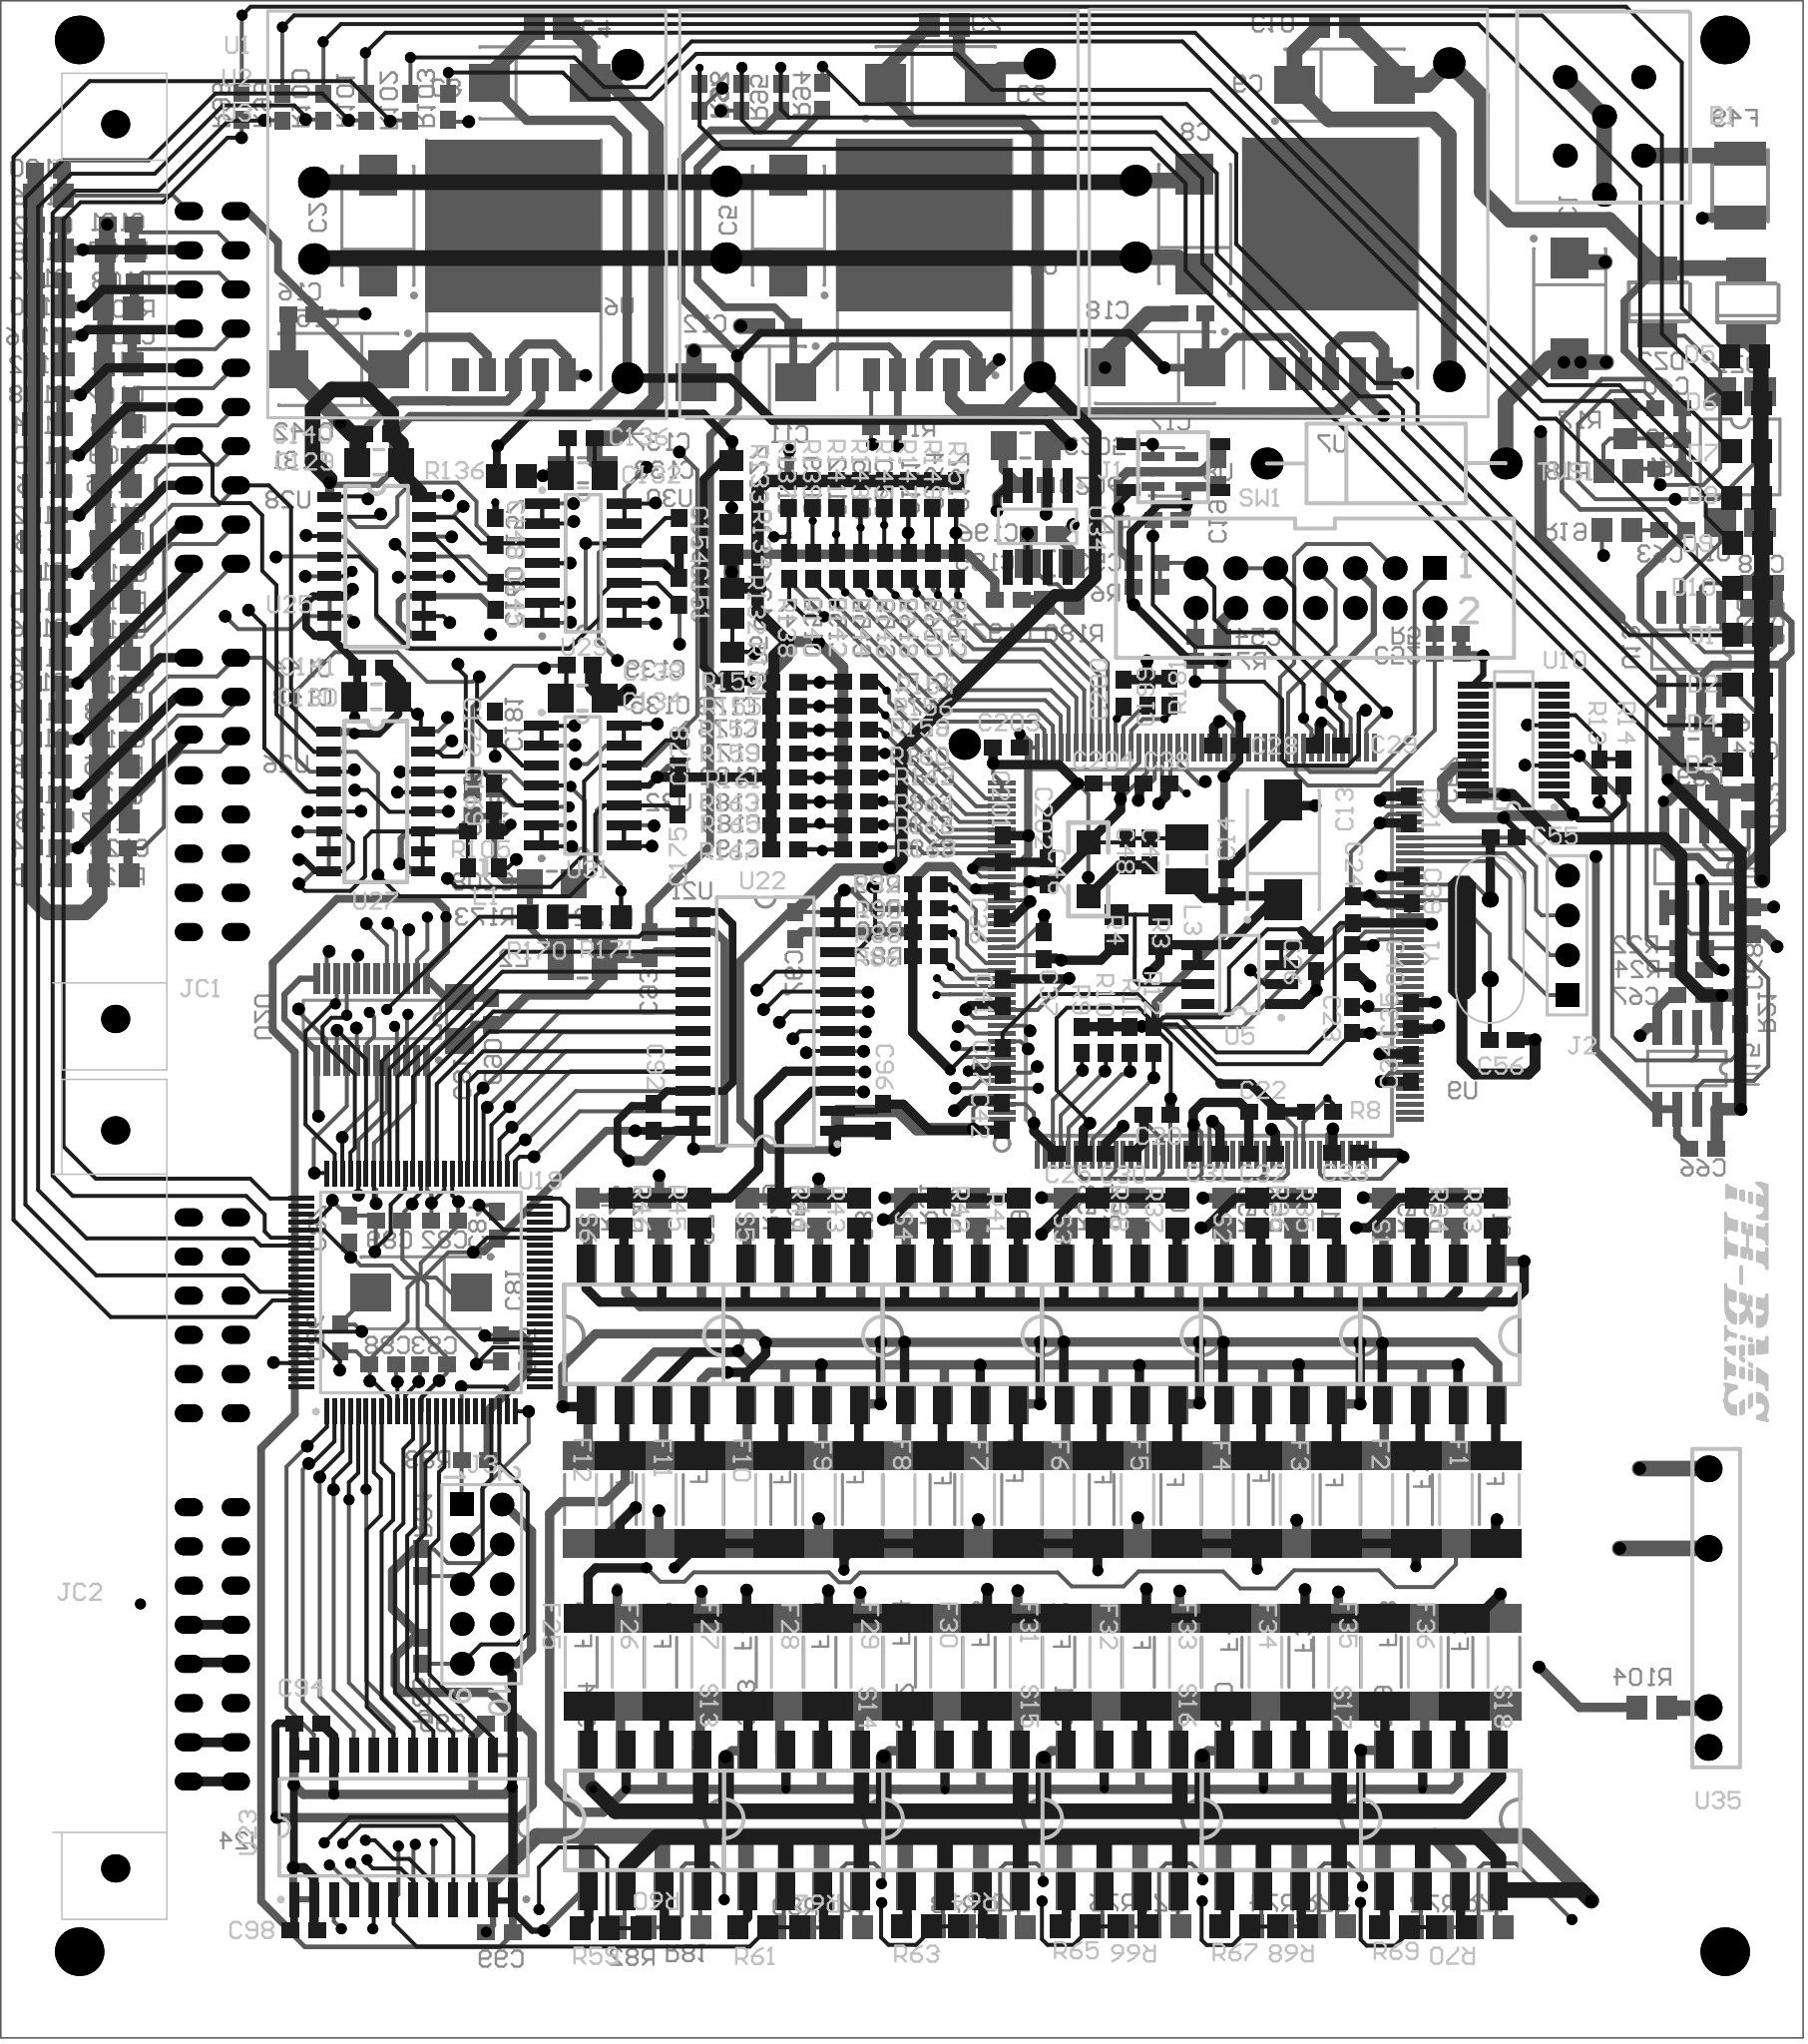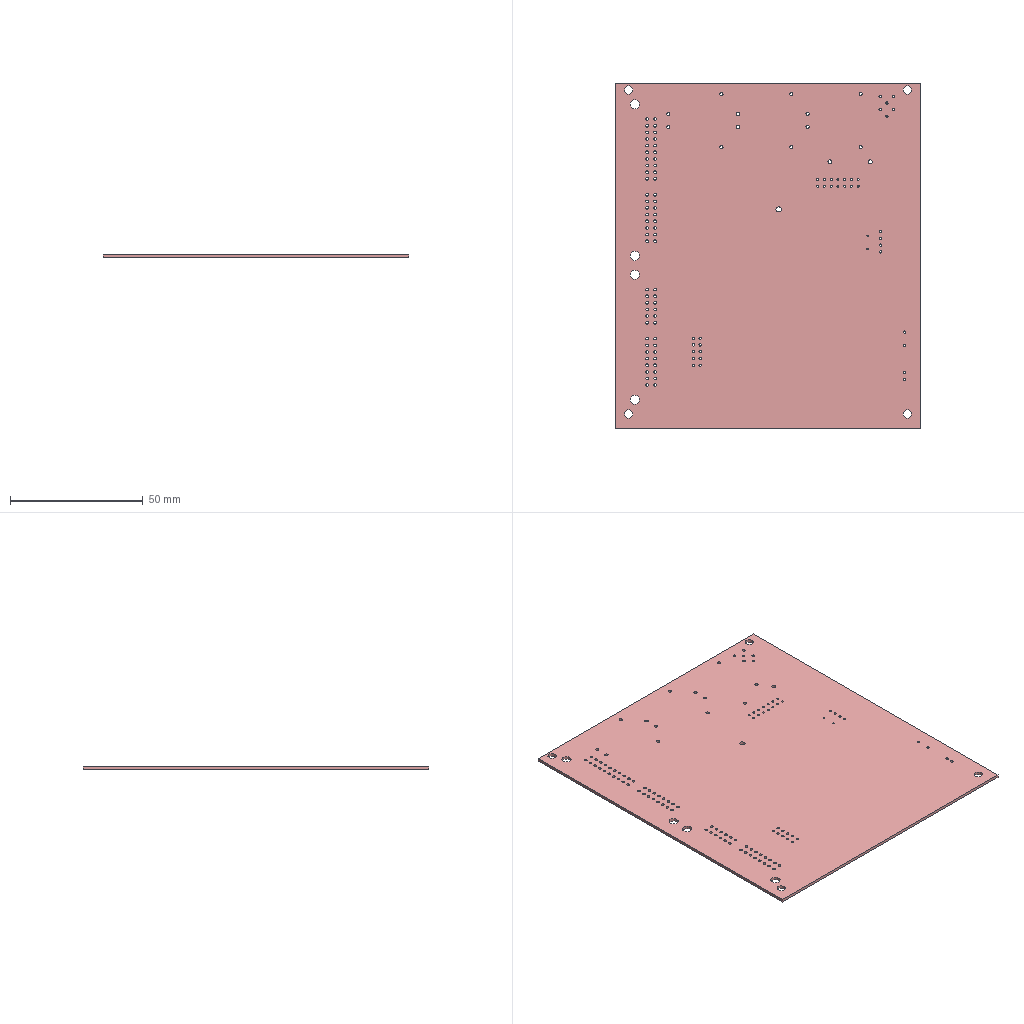Circuit board layout | Altium Designer | box 115 x 130 x 1.1 mm
Layer stack:
# Altium Designer layer stack of  (unit mm; dielectric type: 0 none, 1 core, 2 prepreg, 3 surface material)
index,name,kind,layer,copper_thickness_mm,dielectric_type,dielectric_thickness_mm,dielectric_material,dielectric_constant
0,Top Paste,other,,,,,,
1,Top Overlay,other,,,,,,
2,Top Solder,dielectric,,,3,0.0102,Solder Resist,3.5
3,Top Layer,copper,Top Layer,0.0356,,,,
4,Dielectric1,dielectric,,,1,0.32,FR-4,4.8
5,GND,copper,GND,0.0356,,,,
6,Dielectric2,dielectric,,,2,0.32,FR-4,4.8
7,POWER,copper,POWER,0.0356,,,,
8,Dielectric3,dielectric,,,1,0.32,FR-4,4.8
9,Bottom Layer,copper,Bottom Layer,0.0356,,,,
10,Bottom Solder,dielectric,,,3,0.0102,Solder Resist,3.5
11,Bottom Overlay,other,,,,,,
12,Bottom Paste,other,,,,,,
# drill layer pairs: low layer,high layer
drill_pair,Top Layer,Bottom Layer
Part placement:
Designator,Comment,Layer,Footprint,Center-X(mm),Center-Y(mm),Rotation
D1,RED,TopLayer,CR2012-0805,111.489,85.962,360
D2,RED,TopLayer,CR2012-0805,111.489,82.792,360
D3,GREEN,TopLayer,CR2012-0805,111.459,77.682,360
D4,GREEN,TopLayer,CR2012-0805,111.489,80.222,360
D5,BLUE,TopLayer,CR2012-0805,111.299,103.772,360
D6,BLUE,TopLayer,CR2012-0805,111.389,100.752,360
D7,BLUE,TopLayer,CR2012-0805,111.409,97.732,360
D8,BLUE,TopLayer,CR2012-0805,111.429,94.742,360
D9,BLUE,TopLayer,CR2012-0805,111.449,91.842,360
D10,RED,TopLayer,CR2012-0805,111.469,88.952,360
C55,Cap,TopLayer,CR1608-0603,95.9,73.062,180
C56,Cap,TopLayer,CR1608-0603,95.84,60.138,180
C199,Cap,TopLayer,CR1608-0603,73.152,82.3,270
C35,Cap,TopLayer,CR1608-0603,89.968,61.67,90
R181,Res2,TopLayer,CR1608-0603,74.548,82.32,90
C34,Cap,TopLayer,CR1608-0603,89.982,58.33,270
C38,Cap,TopLayer,CR1608-0603,73.74,76.502,360
R168,Res2,TopLayer,CR1608-0603,54.59,72.32,180
R166,Res2,TopLayer,CR1608-0603,54.59,73.844,180
R164,Res2,TopLayer,CR1608-0603,54.59,75.368,180
R162,Res2,TopLayer,CR1608-0603,54.59,76.892,180
R160,Res2,TopLayer,CR1608-0603,54.59,78.416,180
R158,Res2,TopLayer,CR1608-0603,54.59,79.94,180
R156,Res2,TopLayer,CR1608-0603,54.59,81.464,180
R154,Res2,TopLayer,CR1608-0603,54.59,82.988,180
R152,Res2,TopLayer,CR1608-0603,60.988,90.382,90
R150,Res2,TopLayer,CR1608-0603,59.464,90.382,90
R148,Res2,TopLayer,CR1608-0603,57.94,90.382,90
R146,Res2,TopLayer,CR1608-0603,56.416,90.382,90
R144,Res2,TopLayer,CR1608-0603,54.892,90.382,90
R142,Res2,TopLayer,CR1608-0603,53.368,90.382,90
R140,Res2,TopLayer,CR1608-0603,51.844,90.382,90
R138,Res2,TopLayer,CR1608-0603,50.32,90.382,90
C13,Cap Pol3,TopLayer,TC7343-2917,81.848,72.256,90
C14,Cap,TopLayer,CR1608-0603,78.212,70.17,270
R3,Res2,TopLayer,CR2012-0805,73.972,67.181,270
U22,SN74LVC4245PW,TopLayer,WSO24,48.792,61.314,90
B1,BNX012H,TopLayer,BNX012H,102.31,117.82,270
C20,Cap,TopLayer,CR1608-0603,73.79,55.372,360
C21,Cap,TopLayer,CR1608-0603,89.832,74.83,270
C22,Cap,TopLayer,CR1608-0603,80.51,55.542,360
C23,Cap,TopLayer,CR1608-0603,86.232,61.41,270
C24,Cap,TopLayer,CR1608-0603,86.262,68.45,270
C25,Cap,TopLayer,CR1608-0603,68.23,52.862,360
C26,Cap,TopLayer,CR1608-0603,83.928,65.35,90
C27,Cap,TopLayer,CR1608-0603,63.928,58.76,90
C28,Cap,TopLayer,CR1608-0603,78.25,78.902,360
C29,Cap,TopLayer,CR1608-0603,84.69,78.922,360
C30,Cap,TopLayer,CR1608-0603,71.37,52.868,180
C31,Cap,TopLayer,CR1608-0603,76.95,52.902,360
C32,Cap,TopLayer,CR1608-0603,80.49,52.902,360
C33,Cap,TopLayer,CR1608-0603,85.81,52.908,180
C36,Cap,TopLayer,CR1608-0603,63.882,68.762,270
C37,Cap,TopLayer,CR1608-0603,66.568,66.16,90
C39,Cap,TopLayer,CR1608-0603,90.058,69.72,90
C40,Cap,TopLayer,CR1608-0603,86.258,65.32,90
C41,Cap,TopLayer,CR1608-0603,63.918,63.174,90
C42,Cap,TopLayer,CR1608-0603,63.908,55.26,90
C46,Cap,TopLayer,1206,69.4,71.022,90
C47,Cap,TopLayer,CR1608-0603,73.308,72.13,90
C48,Cap,TopLayer,CR1608-0603,71.888,72.15,90
C92,Cap,TopLayer,CR1608-0603,41.662,55.18,270
C94,Cap,TopLayer,CR1608-0603,19.58,16.528,180
C96,Cap,TopLayer,CR1608-0603,56.272,55.18,270
C98,Cap,TopLayer,CR1608-0603,19.33,3.308,180
C129,Cap,TopLayer,CR3216-1206,24.139,96.992,360
C130,Cap,TopLayer,CR3216-1206,23.981,82.006,360
C132,Cap,TopLayer,CR3216-1206,37.165,96.162,180
C134,Cap,TopLayer,CR3216-1206,37.125,81.976,180
C136,Cap,TopLayer,CR1608-0603,37.054,98.564,180
C138,Cap,TopLayer,CR1608-0603,36.944,84.048,180
C140,Cap,TopLayer,CR1608-0603,24.07,98.798,360
C141,Cap,TopLayer,CR1608-0603,23.61,83.872,360
C145,Cap,TopLayer,CR1608-0603,31.604,88.426,90
C148,Cap,TopLayer,CR1608-0603,31.568,92.588,270
C151,Cap,TopLayer,CR1608-0603,43.282,88.746,270
C154,Cap,TopLayer,CR1608-0603,43.288,92.588,90
C169,Cap,TopLayer,CR1608-0603,31.488,75.66,90
C172,Cap,TopLayer,CR1608-0603,31.512,80.21,270
C175,Cap,TopLayer,CR1608-0603,43.212,75.36,270
C178,Cap,TopLayer,CR1608-0603,43.248,78.402,90
C200,Cap,TopLayer,CR1608-0603,71.672,82.28,270
C201,Cap,TopLayer,CR1608-0603,63.918,72.318,90
C202,Cap,TopLayer,CR1608-0603,66.792,70.89,270
C203,Cap,TopLayer,CR1608-0603,64.17,78.802,360
C204,Cap,TopLayer,CR1608-0603,70.61,76.492,360
F1,Res2,TopLayer,CR6332-2512,95.396,30.806,90
F2,Res2,TopLayer,CR6332-2512,90.316,30.806,90
F3,Res2,TopLayer,CR6332-2512,85.236,30.806,90
F4,Res2,TopLayer,CR6332-2512,80.156,30.806,90
F5,Res2,TopLayer,CR6332-2512,75.076,30.806,90
F6,Res2,TopLayer,CR6332-2512,69.996,30.806,90
F7,Res2,TopLayer,CR6332-2512,64.916,30.806,90
F8,Res2,TopLayer,CR6332-2512,59.836,30.806,90
F9,Res2,TopLayer,CR6332-2512,54.756,30.806,90
F10,Res2,TopLayer,CR6332-2512,49.676,30.806,90
F11,Res2,TopLayer,CR6332-2512,44.596,30.806,90
F12,Res2,TopLayer,CR6332-2512,39.516,30.806,90
F25,Res2,TopLayer,CR6332-2512,37.524,20.42,270
F26,Res2,TopLayer,CR6332-2512,42.604,20.42,270
F27,Res2,TopLayer,CR6332-2512,47.684,20.42,270
F28,Res2,TopLayer,CR6332-2512,52.764,20.42,270
F29,Res2,TopLayer,CR6332-2512,57.844,20.42,270
F30,Res2,TopLayer,CR6332-2512,62.924,20.42,270
F31,Res2,TopLayer,CR6332-2512,68.004,20.42,270
F32,Res2,TopLayer,CR6332-2512,73.084,20.42,270
F33,Res2,TopLayer,CR6332-2512,78.164,20.42,270
F34,Res2,TopLayer,CR6332-2512,83.244,20.42,270
F35,Res2,TopLayer,CR6332-2512,88.324,20.42,270
F36,Res2,TopLayer,CR6332-2512,93.404,20.42,270
J1,JTAG_335,TopLayer,JTAG14,83.866,88.963,180
J2,Header 4,TopLayer,HDR1X4,99.95,66.81,90
J3,JTAG_CPLD,TopLayer,HDR2X5,30.695,25.405,270
JC1,AMP-36P,TopLayer,36P,11.16,90.022,180
JC2,AMP-28P,TopLayer,28P,11.16,30.814,180
L3,Inductor,TopLayer,CR3225-1210,75.705,71.635,90
R4,Res2,TopLayer,CR2012-0805,71.188,67.169,90
R8,Res2,TopLayer,CR1608-0603,84.16,55.548,180
R9,Res2,TopLayer,CR1608-0603,68.998,60.126,90
R10,Res2,TopLayer,CR1608-0603,70.522,60.126,90
R11,Res2,TopLayer,CR1608-0603,72.046,60.126,90
R12,Res2,TopLayer,CR1608-0603,73.57,60.126,90
R13,Res2,TopLayer,CR1608-0603,102.022,77.21,270
R14,Res2,TopLayer,CR1608-0603,103.568,77.21,90
R33,Res2,TopLayer,CR2012-0805,95.414,49.103,90
R34,Res2,TopLayer,CR2012-0805,90.334,49.103,90
R35,Res2,TopLayer,CR2012-0805,84.746,49.103,90
R36,Res2,TopLayer,CR2012-0805,80.174,49.103,90
R37,Res2,TopLayer,CR2012-0805,75.094,49.103,90
R38,Res2,TopLayer,CR2012-0805,70.014,49.103,90
R41,Res2,TopLayer,CR2012-0805,64.934,49.103,90
R42,Res2,TopLayer,CR2012-0805,59.854,49.103,90
R43,Res2,TopLayer,CR2012-0805,54.774,49.103,90
R44,Res2,TopLayer,CR2012-0805,49.694,49.103,90
R45,Res2,TopLayer,CR2012-0805,44.614,49.103,90
R46,Res2,TopLayer,CR2012-0805,39.534,49.103,90
R59,Res2,TopLayer,CR2012-0805,37.899,3.452,360
R60,Res2,TopLayer,CR2012-0805,41.791,3.478,180
R61,Res2,TopLayer,CR2012-0805,47.969,3.502,360
R62,Res2,TopLayer,CR2012-0805,51.941,3.498,180
R63,Res2,TopLayer,CR2012-0805,58.429,3.562,360
R64,Res2,TopLayer,CR2012-0805,62.051,3.548,180
R65,Res2,TopLayer,CR2012-0805,68.579,3.562,360
R66,Res2,TopLayer,CR2012-0805,72.261,3.568,180
R67,Res2,TopLayer,CR2012-0805,78.729,3.552,360
R68,Res2,TopLayer,CR2012-0805,82.431,3.558,180
R69,Res2,TopLayer,CR2012-0805,88.939,3.512,360
R70,Res2,TopLayer,CR2012-0805,92.561,3.538,180
R86,Res2,TopLayer,CR1608-0603,59.05,65.482,360
R88,Res2,TopLayer,CR1608-0603,59.05,67.006,360
R90,Res2,TopLayer,CR1608-0603,59.05,68.53,360
R92,Res2,TopLayer,CR1608-0603,59.05,70.054,360
R131,Res2,TopLayer,CR2012-0805,46.686,83.951,90
R132,Res2,TopLayer,CR2012-0805,46.686,88.015,90
R133,Res2,TopLayer,CR2012-0805,46.65,96.125,270
R134,Res2,TopLayer,CR2012-0805,46.65,92.061,270
R136,Res2,TopLayer,CR2012-0805,32.611,96.126,360
R137,Res2,TopLayer,CR1608-0603,50.284,94.954,270
R139,Res2,TopLayer,CR1608-0603,51.808,94.954,270
R141,Res2,TopLayer,CR1608-0603,53.332,94.954,270
R143,Res2,TopLayer,CR1608-0603,54.856,94.954,270
R145,Res2,TopLayer,CR1608-0603,56.38,94.954,270
R147,Res2,TopLayer,CR1608-0603,57.904,94.954,270
R149,Res2,TopLayer,CR1608-0603,59.428,94.954,270
R151,Res2,TopLayer,CR1608-0603,60.952,94.954,270
R153,Res2,TopLayer,CR1608-0603,50.018,82.952,360
R155,Res2,TopLayer,CR1608-0603,50.018,81.428,360
R157,Res2,TopLayer,CR1608-0603,50.018,79.904,360
R159,Res2,TopLayer,CR1608-0603,50.018,78.38,360
R161,Res2,TopLayer,CR1608-0603,50.018,76.856,360
R163,Res2,TopLayer,CR1608-0603,50.018,75.332,360
R165,Res2,TopLayer,CR1608-0603,50.018,73.808,360
R167,Res2,TopLayer,CR1608-0603,50.018,72.284,360
R170,Res2,TopLayer,CR2012-0805,34.583,67.992,360
R171,Res2,TopLayer,CR2012-0805,38.647,67.992,360
S1,AQW214,TopLayer,AQW214,91.776,41.347,270
S2,AQW214,TopLayer,AQW214,81.617,41.347,270
S3,AQW214,TopLayer,AQW214,71.457,41.347,270
S4,AQW214,TopLayer,AQW214,61.297,41.347,270
S5,AQW214,TopLayer,AQW214,51.136,41.347,270
S6,AQW214,TopLayer,AQW214,40.977,41.347,270
S13,AQW214,TopLayer,AQW214,41.144,10.329,90
S14,AQW214,TopLayer,AQW214,51.303,10.329,90
S15,AQW214,TopLayer,AQW214,61.464,10.329,90
S16,AQW214,TopLayer,AQW214,71.624,10.329,90
S17,AQW214,TopLayer,AQW214,81.784,10.329,90
S18,AQW214,TopLayer,AQW214,91.944,10.329,90
SW1,SW-PB,TopLayer,SW_RESET,74.809,96.694,360
TVS1,1.5KE30A,TopLayer,SB560,88.405,96.92,180
U1,1205,TopLayer,DCDC_5W,29.981,112.368,0
U2,1205,TopLayer,DCDC_5W,56.271,112.428,0
U3,1205,TopLayer,DCDC_5W,82.405,112.478,0
U5,TPS76801Q,TopLayer,D008,79.038,64.305,90
U10,SN74CBTD3384DBLE,TopLayer,DBQ024,96.546,79.258,90
U19,EPM240T100C5N,TopLayer,TQFP100,26.816,44.014,90
U23,SN74LVC4245PW,TopLayer,WSO24,25.71,9.88,360
U25,MAX4619,TopLayer,SO16,23.991,90.355,0
U27,MAX4619,TopLayer,SO16,23.934,75.342,0
U29,OPA4350,TopLayer,751A-02,37.179,90.551,270
U31,OPA4350,TopLayer,751A-02,37.139,76.365,270
U34,ADR420,TopLayer,SO-G8,66.158,92.907,180
U35,AQZ102,TopLayer,AQZ102,108.956,23.875,90
Y1,30M,TopLayer,Oscillator,94.131,66.55,270
R105,Res2,TopLayer,CR1608-0603,30.66,73.448,180
L1,Inductor,TopLayer,INDC2012-0805,30.815,71.108,180
C192,Cap,BottomLayer,CR1608-0603,54.59,72.32,360
C189,Cap,BottomLayer,CR1608-0603,54.59,73.844,360
C186,Cap,BottomLayer,CR1608-0603,54.59,75.368,360
C183,Cap,BottomLayer,CR1608-0603,54.59,76.892,360
C180,Cap,BottomLayer,CR1608-0603,54.59,78.416,360
C177,Cap,BottomLayer,CR1608-0603,54.59,79.94,360
C174,Cap,BottomLayer,CR1608-0603,54.59,81.464,360
C171,Cap,BottomLayer,CR1608-0603,54.59,82.988,360
C168,Cap,BottomLayer,CR1608-0603,60.988,90.382,270
C165,Cap,BottomLayer,CR1608-0603,59.464,90.382,270
C162,Cap,BottomLayer,CR1608-0603,57.94,90.382,270
C159,Cap,BottomLayer,CR1608-0603,56.416,90.382,270
C156,Cap,BottomLayer,CR1608-0603,54.892,90.382,270
C153,Cap,BottomLayer,CR1608-0603,53.368,90.382,270
C150,Cap,BottomLayer,CR1608-0603,51.844,90.382,270
C147,Cap,BottomLayer,CR1608-0603,50.32,90.382,270
C89,Cap,BottomLayer,CR1608-0603,24.784,48.604,360
C81,Cap Pol3,BottomLayer,TC7343-2917,26.81,43.996,180
C82,Cap,BottomLayer,CR1608-0603,28.34,48.604,360
C87,Cap,BottomLayer,CR1608-0603,22.262,48.078,270
U21,SN74LVC4245PW,BottomLayer,WSO24,48.792,61.314,270
C15,Cap Pol3,BottomLayer,TC7343-2917,21.544,102.922,180
C16,Cap,BottomLayer,CR1608-0603,19.19,106.458,360
C17,Cap Pol3,BottomLayer,TC7343-2917,73.664,103.032,180
C18,Cap,BottomLayer,CR1608-0603,76.04,106.468,360
C19,Cap,BottomLayer,CR1608-0603,77.672,96.376,270
C52,Cap,BottomLayer,CR1608-0603,92.36,84.762,180
C53,Cap,BottomLayer,CR1608-0603,73.122,90.556,360
C54,Cap,BottomLayer,CR1608-0603,77.1,85.892,180
C58,Cap,BottomLayer,CR1608-0603,112.4,89.272,180
C59,Cap,BottomLayer,CR1608-0603,113.218,86.84,270
C60,Cap,BottomLayer,CR1608-0603,106.46,100.462,180
C61,Cap,BottomLayer,CR1608-0603,106.52,96.582,180
C62,Cap,BottomLayer,CR1608-0603,106.46,98.422,180
C63,Cap,BottomLayer,CR1608-0603,106.69,92.65,180
C83,Cap,BottomLayer,CR1608-0603,27.61,39.448,360
C84,Cap,BottomLayer,CR1608-0603,31.678,48.32,270
C85,Cap,BottomLayer,CR1608-0603,31.914,40.458,270
C86,Cap,BottomLayer,CR1608-0603,21.658,41.12,270
C88,Cap,BottomLayer,CR1608-0603,24.38,39.422,180
C90,Cap,BottomLayer,CR1608-0603,31.288,61.966,90
C91,Cap,BottomLayer,CR3216-1206,29.256,61.467,90
DZ1,SMBJ8.5CA,BottomLayer,AK_1B,111.36,107.171,180
DZ2,SMBJ8.5CA,BottomLayer,AK_1B,105.72,107.231,180
R5,Res2,BottomLayer,CR1608-0603,92.33,86.032,180
R6,Res2,BottomLayer,CR1608-0603,73.122,89.032,360
R7,Res2,BottomLayer,CR1608-0603,77.1,84.322,180
R17,Res2,BottomLayer,CR2012-0805,103.672,99.459,90
R18,Res2,BottomLayer,CR2012-0805,103.221,96.462,180
R19,Res2,BottomLayer,CR2012-0805,103.125,92.658,180
R83,Res2,BottomLayer,CR1608-0603,30.26,33.332,180
R84,Res2,BottomLayer,CR1608-0603,26.848,26.77,270
R85,Res2,BottomLayer,CR1608-0603,26.848,21.15,270
R104,Res2,BottomLayer,CR2012-0805,105.361,17.492,180
U8,TPS3823-33,BottomLayer,DBV005,74.587,96.385,90
U11,ZJYS-81R5-2PL,BottomLayer,ZJYS,110.993,97.335,90
U20,SN74CBTD3384DBLE,BottomLayer,DBQ024,23.688,61.442,180
R2,Res2,BottomLayer,CR1608-0603,74.39,93.332,180
C131,Cap,BottomLayer,CR3216-1206,24.129,97.008,360
C142,Cap,BottomLayer,CR1608-0603,24.07,98.834,360
C143,Cap,BottomLayer,CR3216-1206,23.981,82.042,360
C144,Cap,BottomLayer,CR1608-0603,23.59,83.868,360
U26,MAX4619,BottomLayer,SO16,23.941,75.345,180
U28,MAX4619,BottomLayer,SO16,23.998,90.352,180
C1,Cap Pol3,BottomLayer,TC7343-2917,100.118,106.824,270
C2,Cap Pol3,BottomLayer,TC7343-2917,24.072,112.09,90
C3,Cap Pol3,BottomLayer,TC7343-2917,34.386,121.208,360
C4,Cap,BottomLayer,CR2012-0805,34.971,124.712,180
F49,2.6A,BottomLayer,FUSE,110.991,114.649,270
C5,Cap Pol3,BottomLayer,TC7343-2917,50.272,112.1,90
C6,Cap Pol3,BottomLayer,TC7343-2917,59.656,121.228,360
C7,Cap,BottomLayer,CR2012-0805,60.201,124.892,180
C8,Cap Pol3,BottomLayer,TC7343-2917,76.192,112.2,90
C9,Cap Pol3,BottomLayer,TC7343-2917,85.756,121.068,360
C10,Cap,BottomLayer,CR2012-0805,85.131,124.812,180
C93,Cap,BottomLayer,CR1608-0603,41.382,66.18,90
C95,Cap,BottomLayer,CR1608-0603,31.81,16.488,360
C97,Cap,BottomLayer,CR1608-0603,50.692,67.43,90
C99,Cap,BottomLayer,CR1608-0603,31.83,3.208,360
C100,Cap,BottomLayer,CR1608-0603,3.05,115.598,360
C101,Cap,BottomLayer,CR1608-0603,7.66,112.188,360
C102,Cap,BottomLayer,CR1608-0603,3.079,112.136,360
C103,Cap,BottomLayer,CR1608-0603,7.689,108.566,360
C104,Cap,BottomLayer,CR1608-0603,3.12,108.618,360
C105,Cap,BottomLayer,CR1608-0603,7.54,105.018,360
C106,Cap,BottomLayer,CR1608-0603,3.12,105.088,360
C107,Cap,BottomLayer,CR1608-0603,7.44,101.278,360
C108,Cap,BottomLayer,CR1608-0603,3,101.318,360
C109,Cap,BottomLayer,CR1608-0603,7.4,97.418,360
C110,Cap,BottomLayer,CR1608-0603,2.96,97.458,360
C111,Cap,BottomLayer,CR1608-0603,7.4,93.638,360
C112,Cap,BottomLayer,CR1608-0603,2.87,93.608,360
C113,Cap,BottomLayer,CR1608-0603,7.32,89.888,360
C114,Cap,BottomLayer,CR1608-0603,2.89,89.918,360
C115,Cap,BottomLayer,CR1608-0603,7.3,86.25,360
C116,Cap,BottomLayer,CR1608-0603,2.86,86.316,360
C117,Cap,BottomLayer,CR1608-0603,7.25,82.812,360
C118,Cap,BottomLayer,CR1608-0603,2.92,82.898,360
C119,Cap,BottomLayer,CR1608-0603,7.26,79.334,360
C120,Cap,BottomLayer,CR1608-0603,2.94,79.31,360
C121,Cap,BottomLayer,CR1608-0603,7.269,75.814,360
C122,Cap,BottomLayer,CR1608-0603,2.97,75.822,360
C123,Cap,BottomLayer,CR1608-0603,7.28,72.358,360
C124,Cap,BottomLayer,CR1608-0603,2.98,72.398,360
F13,Res2,BottomLayer,CR6332-2512,37.484,30.806,90
F14,Res2,BottomLayer,CR6332-2512,42.056,30.806,90
F15,Res2,BottomLayer,CR6332-2512,47.644,30.806,90
F16,Res2,BottomLayer,CR6332-2512,52.216,30.806,90
F17,Res2,BottomLayer,CR6332-2512,57.804,30.806,90
F18,Res2,BottomLayer,CR6332-2512,62.376,30.806,90
F19,Res2,BottomLayer,CR6332-2512,67.964,30.806,90
F20,Res2,BottomLayer,CR6332-2512,72.536,30.806,90
F21,Res2,BottomLayer,CR6332-2512,78.124,30.806,90
F22,Res2,BottomLayer,CR6332-2512,82.696,30.806,90
F23,Res2,BottomLayer,CR6332-2512,88.284,30.806,90
F24,Res2,BottomLayer,CR6332-2512,92.856,30.806,90
F37,Res2,BottomLayer,CR6332-2512,95.436,20.42,270
F38,Res2,BottomLayer,CR6332-2512,90.864,20.42,270
F39,Res2,BottomLayer,CR6332-2512,85.276,20.42,270
F40,Res2,BottomLayer,CR6332-2512,80.704,20.42,270
F41,Res2,BottomLayer,CR6332-2512,75.116,20.42,270
F42,Res2,BottomLayer,CR6332-2512,70.036,20.42,270
F43,Res2,BottomLayer,CR6332-2512,64.956,20.42,270
F44,Res2,BottomLayer,CR6332-2512,59.876,20.42,270
F45,Res2,BottomLayer,CR6332-2512,54.796,20.42,270
F46,Res2,BottomLayer,CR6332-2512,49.716,20.42,270
F47,Res2,BottomLayer,CR6332-2512,44.636,20.42,270
F48,Res2,BottomLayer,CR6332-2512,39.556,20.42,270
R47,Res2,BottomLayer,CR2012-0805,37.466,49.103,90
R48,Res2,BottomLayer,CR2012-0805,42.038,49.103,90
R49,Res2,BottomLayer,CR2012-0805,47.626,49.103,90
R50,Res2,BottomLayer,CR2012-0805,52.198,49.103,90
R51,Res2,BottomLayer,CR2012-0805,57.786,49.103,90
R52,Res2,BottomLayer,CR2012-0805,62.358,49.103,90
R53,Res2,BottomLayer,CR2012-0805,67.946,49.103,90
R54,Res2,BottomLayer,CR2012-0805,72.518,49.103,90
R55,Res2,BottomLayer,CR2012-0805,78.106,49.103,90
R56,Res2,BottomLayer,CR2012-0805,82.678,49.103,90
R57,Res2,BottomLayer,CR2012-0805,88.266,49.103,90
R58,Res2,BottomLayer,CR2012-0805,92.838,49.103,90
R71,Res2,BottomLayer,CR2012-0805,94.941,3.542,180
R72,Res2,BottomLayer,CR2012-0805,91.089,3.508,360
R73,Res2,BottomLayer,CR2012-0805,84.841,3.592,180
R74,Res2,BottomLayer,CR2012-0805,80.889,3.568,360
R75,Res2,BottomLayer,CR2012-0805,74.341,3.552,180
R76,Res2,BottomLayer,CR2012-0805,70.709,3.548,360
R77,Res2,BottomLayer,CR2012-0805,64.451,3.542,180
R78,Res2,BottomLayer,CR2012-0805,60.589,3.558,360
R79,Res2,BottomLayer,CR2012-0805,54.021,3.532,180
R80,Res2,BottomLayer,CR2012-0805,50.439,3.488,360
R81,Res2,BottomLayer,CR2012-0805,43.751,3.492,180
R82,Res2,BottomLayer,CR2012-0805,40.239,3.498,360
R106,Res2,BottomLayer,CR2012-0805,3.041,114.012,180
R107,Res2,BottomLayer,CR2012-0805,7.651,110.522,180
R108,Res2,BottomLayer,CR2012-0805,3.07,110.51,180
R109,Res2,BottomLayer,CR2012-0805,7.53,106.81,180
R110,Res2,BottomLayer,CR2012-0805,3.111,106.932,180
R111,Res2,BottomLayer,CR2012-0805,7.531,103.272,180
R112,Res2,BottomLayer,CR2012-0805,3.111,103.252,180
R113,Res2,BottomLayer,CR2012-0805,7.431,99.282,180
R114,Res2,BottomLayer,CR2012-0805,2.991,99.422,180
R115,Res2,BottomLayer,CR2012-0805,7.391,95.502,180
R116,Res2,BottomLayer,CR2012-0805,2.951,95.502,180
R117,Res2,BottomLayer,CR2012-0805,7.321,91.922,180
R118,Res2,BottomLayer,CR2012-0805,2.861,91.922,180
R119,Res2,BottomLayer,CR2012-0805,7.311,88.082,180
R120,Res2,BottomLayer,CR2012-0805,2.881,88.172,180
R121,Res2,BottomLayer,CR2012-0805,7.311,84.492,180
R122,Res2,BottomLayer,CR2012-0805,2.901,84.492,180
R123,Res2,BottomLayer,CR2012-0805,7.231,81.122,180
R124,Res2,BottomLayer,CR2012-0805,2.931,81.102,180
R125,Res2,BottomLayer,CR2012-0805,7.271,77.572,180
R126,Res2,BottomLayer,CR2012-0805,2.911,77.582,180
R127,Res2,BottomLayer,CR2012-0805,7.28,74.11,180
R128,Res2,BottomLayer,CR2012-0805,2.951,74.162,180
R129,Res2,BottomLayer,CR2012-0805,7.271,70.642,180
R130,Res2,BottomLayer,CR2012-0805,2.935,70.618,180
S7,AQW214,BottomLayer,AQW214,41.103,41.347,270
S8,AQW214,BottomLayer,AQW214,51.264,41.347,270
S9,AQW214,BottomLayer,AQW214,61.423,41.347,270
S10,AQW214,BottomLayer,AQW214,71.584,41.347,270
S11,AQW214,BottomLayer,AQW214,81.743,41.347,270
S12,AQW214,BottomLayer,AQW214,91.903,41.347,270
S19,AQW214,BottomLayer,AQW214,91.817,10.329,90
S20,AQW214,BottomLayer,AQW214,81.656,10.329,90
S21,AQW214,BottomLayer,AQW214,71.496,10.329,90
S22,AQW214,BottomLayer,AQW214,61.337,10.329,90
S23,AQW214,BottomLayer,AQW214,51.176,10.329,90
S24,AQW214,BottomLayer,AQW214,41.017,10.329,90
U24,SN74LVC4245PW,BottomLayer,WSO24,25.704,9.892,180
C11,Cap Pol3,BottomLayer,TC7343-2917,47.554,102.102,180
C12,Cap,BottomLayer,CR1608-0603,49.73,105.688,360
C133,Cap,BottomLayer,CR3216-1206,37.161,96.482,180
C135,Cap,BottomLayer,CR3216-1206,37.125,81.94,180
C137,Cap,BottomLayer,CR1608-0603,37.054,98.528,180
C139,Cap,BottomLayer,CR1608-0603,36.944,84.012,180
C157,Cap,BottomLayer,CR1608-0603,31.604,92.588,270
C160,Cap,BottomLayer,CR1608-0603,31.568,88.426,90
C163,Cap,BottomLayer,CR1608-0603,43.252,92.588,90
C166,Cap,BottomLayer,CR1608-0603,43.318,88.746,270
C181,Cap,BottomLayer,CR1608-0603,31.524,80.222,270
C184,Cap,BottomLayer,CR1608-0603,31.502,75.32,90
C187,Cap,BottomLayer,CR1608-0603,43.212,78.402,90
R172,Res2,BottomLayer,CR2012-0805,38.629,67.992,180
R173,Res2,BottomLayer,CR2012-0805,34.611,68.052,180
U9,TMS320F283XXPGF_23,BottomLayer,QFP176NEW,76.889,65.793,90
U30,OPA4350,BottomLayer,751A-02,37.179,90.561,90
U32,OPA4350,BottomLayer,751A-02,37.139,76.375,90
C125,Cap,BottomLayer,CR2012-0805,46.686,83.933,270
C126,Cap,BottomLayer,CR2012-0805,46.686,87.997,270
C146,Cap,BottomLayer,CR1608-0603,50.32,94.954,270
C149,Cap,BottomLayer,CR1608-0603,51.844,94.954,270
C152,Cap,BottomLayer,CR1608-0603,53.368,94.954,270
C155,Cap,BottomLayer,CR1608-0603,54.892,94.954,270
C158,Cap,BottomLayer,CR1608-0603,56.416,94.954,270
C161,Cap,BottomLayer,CR1608-0603,57.94,94.954,270
C164,Cap,BottomLayer,CR1608-0603,59.464,94.954,270
C167,Cap,BottomLayer,CR1608-0603,60.988,94.954,270
C170,Cap,BottomLayer,CR1608-0603,50.018,82.988,360
C173,Cap,BottomLayer,CR1608-0603,50.018,81.464,360
C176,Cap,BottomLayer,CR1608-0603,50.018,79.94,360
C179,Cap,BottomLayer,CR1608-0603,50.018,78.416,360
C182,Cap,BottomLayer,CR1608-0603,50.018,76.892,360
C185,Cap,BottomLayer,CR1608-0603,50.018,75.368,360
C188,Cap,BottomLayer,CR1608-0603,50.018,73.844,360
C191,Cap,BottomLayer,CR1608-0603,50.018,72.32,360
R20,Res2,BottomLayer,CR1608-0603,111.508,86.84,270
R22,Res2,BottomLayer,CR1608-0603,107.92,65.982,180
R87,Res2,BottomLayer,CR1608-0603,59.05,65.482,180
R89,Res2,BottomLayer,CR1608-0603,59.05,67.006,180
R91,Res2,BottomLayer,CR1608-0603,59.05,68.53,180
R93,Res2,BottomLayer,CR1608-0603,59.05,70.054,180
R94,Res2,BottomLayer,CR1608-0603,52.442,120.332,90
R95,Res2,BottomLayer,CR1608-0603,49.788,120.302,90
R96,Res2,BottomLayer,CR1608-0603,44.61,120.302,90
R97,Res2,BottomLayer,CR1608-0603,47.256,120.292,90
R98,Res2,BottomLayer,CR1608-0603,15.386,119.704,90
R99,Res2,BottomLayer,CR1608-0603,17.972,119.664,90
R100,Res2,BottomLayer,CR1608-0603,20.598,119.664,90
R101,Res2,BottomLayer,CR1608-0603,23.294,119.664,90
R102,Res2,BottomLayer,CR1608-0603,26.15,119.664,90
R103,Res2,BottomLayer,CR1608-0603,28.556,119.674,90
U13,SN65HVD251,BottomLayer,D008,107.855,85.052,180
U15,HCPL063,BottomLayer,SO-G8,107.596,58.313,180
U16,HCPL063,BottomLayer,SO-G8,108.058,71.191,180
R1,Res2,BottomLayer,CR1608-0603,56.39,99.252,180
C127,Cap,BottomLayer,CR2012-0805,46.65,96.143,90
C128,Cap,BottomLayer,CR2012-0805,46.65,92.079,90
U4,TPS75733,BottomLayer,75733,58.947,107.339,180
U6,TPS75733,BottomLayer,75733,32.747,107.329,180
U7,TPS75733,BottomLayer,75733,84.867,107.439,180
C209,Cap,BottomLayer,CR1608-0603,30.102,75.27,90
C208,Cap,BottomLayer,CR3216-1206,35.169,70.098,360
C57,Cap,BottomLayer,CR1608-0603,93.968,76.68,270
C64,Cap,BottomLayer,CR3216-1206,108.021,78.542,180
C65,Cap,BottomLayer,CR1608-0603,107.8,80.382,180
C66,Cap,BottomLayer,CR1608-0603,108.61,53.218,360
C67,Cap,BottomLayer,CR1608-0603,107.85,62.968,360
C68,Cap,BottomLayer,CR1608-0603,111.802,67.76,90
C69,Cap,BottomLayer,CR1608-0603,108.51,75.928,360
C195,Cap,BottomLayer,CR3216-1206,66.941,90.552,180
C196,Cap,BottomLayer,CR1608-0603,66.42,92.442,180
C197,Cap,BottomLayer,CR1608-0603,64.28,88.228,360
C205,Cap,BottomLayer,CR3216-1206,65.379,98.068,360
C206,Cap,BottomLayer,CR1608-0603,65.84,95.548,360
L2,Inductor,BottomLayer,CR3225-1210,37.125,65.335,180
R21,Res2,BottomLayer,CR1608-0603,110.972,62.02,90
R23,Res2,BottomLayer,CR1608-0603,111.542,75.08,90
R24,Res2,BottomLayer,CR1608-0603,107.87,64.602,180
R180,Res2,BottomLayer,CR2012-0805,67.529,88.038,360
Pad and via stacks:
# Altium Designer via and pad stacks of  (unit mm). Each distinct definition once, with the count of objects using it.
# via: kind,start_layer,end_layer,hole_mm,diameter_mm,mode(0 simple;1 top-mid-bottom;2 full stack),diameter_per_layer,count,example_net
# pad: kind,layer,hole_mm,hole_type(0 round;1 square;2 slot),plating,top_size,top_shape(1 round;2 rect;3 octagon;9 rounded rect),mid_size,bottom_size,mode,footprint,size_per_layer,count,example
pad,Top Layer,0,0,plated,1.5x1.3,2,1.5x1.3,1.5x1.3,0,CR2012-0805,,86,D3.2
pad,Top Layer,0,0,plated,7.874x1.778,3,7.874x1.778,7.874x1.778,0,Oscillator,,1,Y1.3
pad,Top Layer,0,0,plated,1x1.1,2,1x1.1,1x1.1,0,CR1608-0603,,190,C55.1
pad,Top Layer,0,0,plated,2.6x2.4,2,2.6x2.4,2.6x2.4,0,TC7343-2917,,2,C13.1
pad,Top Layer,0,0,plated,2.7x1.6,2,2.7x1.6,2.7x1.6,0,CR3225-1210,,2,L3.1
pad,Top Layer,0,0,plated,0.4x1.95,2,0.4x1.95,0.4x1.95,0,DBQ024,,24,U10.13
pad,Top Layer,0,0,plated,0.6x2.2,2,0.6x2.2,0.6x2.2,0,WSO24,,48,U22.21
pad,Top Layer,0,0,plated,1.5x0.635,2,1.5x0.635,1.5x0.635,0,SO16,,32,U27.2
pad,Top Layer,0,0,plated,1.8x1.6,2,1.8x1.6,1.8x1.6,0,CR3216-1206,,8,C134.2
pad,Top Layer,0,0,plated,3.2x1.8,2,3.2x1.8,3.2x1.8,0,CR6332-2512,,48,F36.2
pad,Top Layer,0,0,plated,2.54x1.143,2,2.54x1.143,2.54x1.143,0,AQW214,,96,S18.1
pad,Top Layer,0,0,plated,0.6x2.2,2,0.6x2.2,0.6x2.2,0,SO-G8,,8,U34.3
pad,Top Layer,0,0,plated,0.6x2.2,2,0.6x2.2,0.6x2.2,0,751A-02,,28,U31.12
pad,Top Layer,0,0,plated,1.6x0.3,2,1.6x0.3,1.6x0.3,0,TQFP100,,100,U19.1
pad,Top Layer,0,0,plated,1.524x1.524,2,1.524x1.524,1.524x1.524,0,1206,,2,C46.2
pad,Top Layer,0,0,plated,1.524x0.762,2,1.524x0.762,1.524x0.762,0,SW_RESET,,4,SW1.4
pad,Top Layer,0,0,plated,0.6x2.05,2,0.6x2.05,0.6x2.05,0,D008,,8,U5.5
pad,Top Layer,0,0,plated,1.2x1,2,1.2x1,1.2x1,0,INDC2012-0805,,2,L1.1
pad,Bottom Layer,0,0,plated,1x1.1,2,1x1.1,1x1.1,0,CR1608-0603,,262,C209.1
pad,Bottom Layer,0,0,plated,1.8x1.6,2,1.8x1.6,1.8x1.6,0,CR3216-1206,,18,C208.2
pad,Bottom Layer,0,0,plated,2.7x1.6,2,2.7x1.6,2.7x1.6,0,CR3225-1210,,2,L2.2
pad,Bottom Layer,0,0,plated,1.5x1.3,2,1.5x1.3,1.5x1.3,0,CR2012-0805,,126,R180.1
pad,Bottom Layer,0,0,plated,1.778x0.3,2,1.778x0.3,1.778x0.3,0,QFP176NEW,,176,U9.53
pad,Bottom Layer,0,0,plated,0.6x2.2,2,0.6x2.2,0.6x2.2,0,WSO24,,48,U21.10
pad,Bottom Layer,0,0,plated,11.176x11,2,11.176x11,11.176x11,0,75733,,3,U7.6
pad,Bottom Layer,0,0,plated,1.05x2.1,2,1.05x2.1,1.05x2.1,0,75733,,15,U7.2
pad,Bottom Layer,0,0,plated,2.6x2.4,2,2.6x2.4,2.6x2.4,0,TC7343-2917,,22,C8.1
pad,Bottom Layer,0,0,plated,1.5x0.635,2,1.5x0.635,1.5x0.635,0,SO16,,32,U28.13
pad,Bottom Layer,0,0,plated,0.6x2.2,2,0.6x2.2,0.6x2.2,0,SO-G8,,16,U16.1
pad,Bottom Layer,0,0,plated,0.6x2.05,2,0.6x2.05,0.6x2.05,0,D008,,8,U13.1
pad,Bottom Layer,0,0,plated,0.6x2.2,2,0.6x2.2,0.6x2.2,0,751A-02,,28,U32.11
pad,Bottom Layer,0,0,plated,2.54x1.143,2,2.54x1.143,2.54x1.143,0,AQW214,,96,S24.8
pad,Bottom Layer,0,0,plated,3.2x1.8,2,3.2x1.8,3.2x1.8,0,CR6332-2512,,48,F48.1
pad,Bottom Layer,0,0,plated,1.524x3.302,2,1.524x3.302,1.524x3.302,0,FUSE,,2,F49.2
pad,Bottom Layer,0,0,plated,0.55x1.45,2,0.55x1.45,0.55x1.45,0,DBV005,,5,U8.1
pad,Bottom Layer,0,0,plated,0.4x1.95,2,0.4x1.95,0.4x1.95,0,DBQ024,,24,U20.1
pad,Bottom Layer,0,0,plated,1.524x2.54,2,1.524x2.54,1.524x2.54,0,AK_1B,,4,DZ2.2
pad,Bottom Layer,0,0,plated,1.8x2,2,1.8x2,1.8x2,0,ZJYS,,4,U11.4
pad,Multi-Layer,0.762,0,plated,1.524x1.524,1,1.524x1.524,1.524x1.524,0,JTAG14,,13,J1.7
pad,Multi-Layer,0.762,0,plated,1.524x1.524,2,1.524x1.524,1.524x1.524,0,JTAG14,,1,J1.1
pad,Multi-Layer,0.508,0,plated,1.016x1.016,1,1.016x1.016,1.016x1.016,0,Oscillator,,2,Y1.1
pad,Multi-Layer,1.2,0,plated,2x2,1,2x2,2x2,0,DCDC_5W,,12,U3.1
pad,Multi-Layer,1.397,0,plated,2.032x2.032,1,2.032x2.032,2.032x2.032,0,SB560,,2,TVS1.2
pad,Multi-Layer,1,0,plated,1.524x1.524,1,1.524x1.524,1.524x1.524,0,BNX012H,,4,B1.1
pad,Multi-Layer,0.9,0,plated,1.7x1.7,1,1.7x1.7,1.7x1.7,0,AQZ102,,4,U35.4
pad,Multi-Layer,0.9,0,plated,1.5x1.5,2,1.5x1.5,1.5x1.5,0,HDR1X4,,1,J2.1
pad,Multi-Layer,0.9,0,plated,1.5x1.5,1,1.5x1.5,1.5x1.5,0,HDR1X4,,3,J2.2
pad,Multi-Layer,0.9,0,plated,1.5x1.5,2,1.5x1.5,1.5x1.5,0,HDR2X5,,1,J3.1
pad,Multi-Layer,0.9,0,plated,1.5x1.5,1,1.5x1.5,1.5x1.5,0,HDR2X5,,9,J3.2
pad,Multi-Layer,0.8,0,plated,1.524x1.524,1,1.524x1.524,1.524x1.524,0,BNX012H,,2,B1.5
pad,Multi-Layer,3.1,0,plated,3.1x3.1,1,3.1x3.1,3.1x3.1,0,,,4,1
pad,Multi-Layer,1,0,plated,1.8x1.143,1,1.8x1.143,1.8x1.143,0,28P,,28,JC2.3
pad,Multi-Layer,3.5,0,plated,1.8x1.8,1,1.8x1.8,1.8x1.8,0,28P,,2,JC2.0
pad,Multi-Layer,1,0,plated,1.8x1.143,1,1.8x1.143,1.8x1.143,0,36P,,36,JC1.17
pad,Multi-Layer,3.5,0,plated,1.8x1.8,1,1.8x1.8,1.8x1.8,0,36P,,2,JC1.0
pad,Multi-Layer,2,0,plated,2x2,1,2x2,2x2,0,,,1,5
via,Top Layer,Bottom Layer,0.4,0.7,0,,83,BAT23
via,Top Layer,Bottom Layer,0.4,0.8,0,,339,BAT8
via,Top Layer,Bottom Layer,0.254,0.5,0,,37,NetC200_2
Copper pours:
name,layer,net,type(0 solid;1 hatched;2 none)
Top Layer-No Net,GND,GNDA,0
Top Layer-No Net,POWER,GNDD,0
Design rules, without the lines most boards share:
# Altium Designer design rules of  (exported by Altium Designer, unit mm)
# columns: name | kind | enabled | priority | scope1 | scope2 | descriptor | typed fields (field=value)
PlaneClearance | 12 | enabled | 1 | All | All | Power Plane Clearance (Clearance =0.508mm) (All) | clearance=0.508
PolygonConnect | 20 | enabled | 1 | All | All | Polygon Connect Rule(Relief Connect )(Conductor Width=0.254mm) (Relief Angle=90 Angle) (Entries=4) (Air Gap Width=0.254mm) (All),(All) | connect_style(0=relief,1=direct,2=none)=0 relief_conductor_width=0.254 relief_entries=4
PasteMaskExpansion | 14 | enabled | 1 | All | All | Paste Mask Expansion (Expansion =0mm) (All) | expansion=0
SolderMaskExpansion | 13 | enabled | 1 | All | All | Solder Mask Expansion (Expansion =0.102mm) (All) | expansion=0.1016
TestPointUsage | 44 | enabled | 1 | All | All | Fabrication Testpoint Usage (Valid =One Required, Allow multiple per net=No) (All) |
Testpoint | 43 | enabled | 1 | All | All | Fabrication Testpoint Style (Under Component=Yes) (All) |
ComponentClearance | 24 | enabled | 1 | All | All | Component Clearance Constraint ( Horizontal Gap = 0.254mm, Vertical Gap = 0.254mm ) (All),(All)  | gap=0.254
Height | 50 | enabled | 1 | All | All | Height Constraint (Min=0mm) (Max=25.4mm) (Prefered=12.7mm) (All) | min_height=0 max_height=25.4
HoleSize | 42 | enabled | 1 | All | All | Hole Size Constraint (Min=0.025mm) (Max=2.54mm) (All) |
Width | 2 | enabled | 1 | All | All | Width Constraint (Min=0.254mm) (Max=254mm) (Preferred=0.254mm) (All) |
Clearance | 0 | enabled | 1 | All | All | Clearance Constraint (Gap=0.3mm) (All),(All) | gap=0.3
RoutingCorners | 10 | enabled | 1 | All | All | Routing Corners (Style=45-Degree) (Min Setback=2.54mm) (Max Setback=2.54mm) (All) |
RoutingVias | 11 | enabled | 1 | All | All | Routing Via (MinHoleWidth=0.305mm) (MaxHoleWidth=5.08mm) (PreferredHoleWidth=0.381mm) (MinWidth=0.559mm) (MaxWidth=6.858mm) (PreferedWidth=0.762mm) (All) | via_min_hole=0.3048 via_max_hole=5.08 via_preferred_diameter=0.762 via_preferred_hole=0.381
PlaneConnect | 6 | enabled | 1 | All | All | Power Plane Connect Rule(Relief Connect )(Expansion=0.508mm) (Conductor Width=0.254mm) (Air Gap=0.254mm) (Entries=4) (All) | relief_conductor_width=0.254 relief_entries=4 relief_expansion=0.508
DiffPairsRouting | 51 | enabled | 1 | All | All | Differential Pairs Uncoupled Length using the Gap Constraints (Min=0.254mm) (Max=0.254mm) (Prefered=0.254mm)  and Width Constraints (Min=0.381mm) (Max=0.381mm) (Prefered=0.381mm) (All) |
HoleToHoleClearance | 52 | enabled | 1 | All | All | Hole To Hole Clearance (Gap=0.254mm) (All),(All) | gap=0.254
MinimumSolderMaskSliver | 53 | enabled | 1 | All | All | Minimum Solder Mask Sliver (Gap=0.254mm) (All),(All) |
SilkscreenOverComponentPads | 54 | enabled | 1 | IsPad | All | Silk To Solder Mask (Clearance=0.254mm) (IsPad),(All) |
SilkToSilkClearance | 55 | enabled | 1 | All | All | Silk to Silk (Clearance=0.254mm) (All),(All) |
NetAntennae | 56 | enabled | 1 | All | All | Net Antennae (Tolerance=0mm) (All) |
Classes set for this board:
# Altium Designer classes of  (member kind: 0 net, 1 component, 2 from-to, 3 pad, 4 layer, 5 differential pair, 6 design channel, 7 polygon, 8 structure, 9 xSignal)
# columns: class name | member kind | superclass | members
BSM4 | 1 | no | B1; C1; C2; C3; C4; C5; C6; C7; C8; C9; C10; C11; C12; C13; C14; C15; C16; C17; C18; C19; C20; C21; C22; C23; C24; C25; C26; C27; C28; C29; C30; C31; C32; C33; C34; C35; C36; C37; C38; C39; C40; C41; C42; C46; C47; C48; C52; C53; C54; C55; C56; C57; C58; C59; C60; C61; C62; C63; C64; C65; C66; C67; C68; C69; C81; C82; C83; C84; C85; C86; C87; C88; C89; C90; C91; C92; C93; C94; C95; C96; C97; C98; C99; C100; C101; C102; C103; C104; C105; C106; C107; C108; C109; C110; C111; C112; C113; C114; C115; C116; C117; C118; C119; C120; C121; C122; C123; C124; C125; C126; C127; C128; C129; C130; C131; C132; C133; C134; C135; C136; C137; C138; C139; C140; C141; C142; C143; C144; C145; C146; C148; C149; C151; C152; C154; C155; C157; C158; C160; C161; C163; C164; C166; C167; C169; C170; C172; C173; C175; C176; C178; C179; C181; C182; C184; C185; C187; C188; C191; C195; C196; C197; C199; C200; C201; C202; C203; C204; C205; C206; D1; D2; D3; D4; D5; D6; D7; D8; D9; D10; DZ1; DZ2; F1; F2; F3; F4; F5; F6; F7; F8; F9; F10; F11; F12; F13; F14; F15; F16; F17; F18; F19; F20; F21; F22; F23; F24; F25; F26; F27; F28; F29; F30; F31; F32; F33; F34; F35; F36; F37; F38; F39; F40; F41; F42; F43; F44; F45; F46; F47; F48; F49; J1; J2; J3; JC1; JC2; L2; L3; R3; R4; R5; R6; R7; R8; R9; R10; R11; R12; R13; R14; R17; R18; R19; R20; R21; R22; R23; R24; R33; R34; R35; R36; R37; R38; R41; R42; R43; R44; R45; R46; R47; R48; R49; R50; R51; R52; R53; R54; R55; R56; R57; R58; R59; R60; R61; R62; R63; R64; R65; R66; R67; R68; R69; R70; R71; R72; R73; R74; R75; R76; R77; R78; R79; R80; R81; R82; R83; R84; R85; R86; R87; R88; R89; R90; R91; R92; R93; R94; R95; R96; R97; R98; R99; R100; R101; R102; R103; R104; R105; R106; R107; R108; R109; R110; R111; R112; R113; R114; R115; R116; R117; R118; R119; R120; R121; R122; R123; R124; R125; R126; R127; R128; R129; R130; R131; R132; R133; R134; R136; R137; R139; R141; R143; R145; R147; R149; R151; R153; R155; R157; R159; R161; R163; R165; R167; R170; R171; R172; R173; R180; R181; S1; S2; S3; S4; S5; S6; S7; S8; S9; S10; S11; S12; S13; S14; S15; S16; S17; S18; S19; S20; S21; S22; S23; S24; SW1; TVS1; U1; U2; U3; U4; U5; U6; U7; U8; U9; U10; U11; U13; U15; U16; U19; U20; U21; U22; U23; U24; U25; U26; U27; U28; U29; U30; U31; U32; U34; U35; Y1; R1; R2; C208; C209; L1; C147; C150; C153; C156; C159; C162; C165; C168; C171; C174; C177; C180; C183; C186; C189; C192; R138; R140; R142; R144; R146; R148; R150; R152; R154; R156; R158; R160; R162; R164; R166; R168;